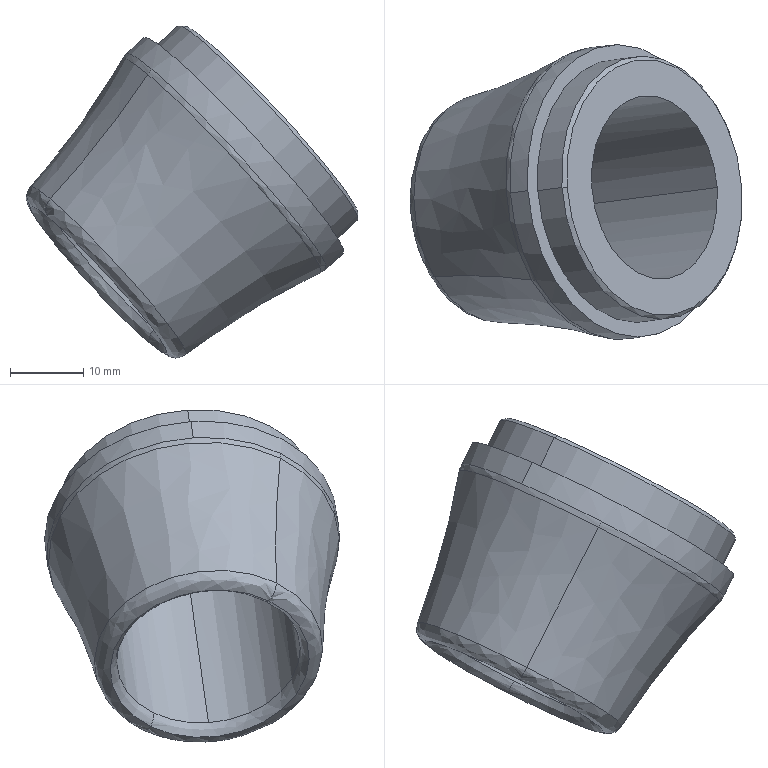Part | SolidWorks | features BaseBody 1 | 1 solid | 18 faces | box 45.199 x 40.143 x 45.272 mm | volume 15779 mm3 | spline 8 | cylinder 4 | cone 4 | plane 2 | commonest cylinder face diameters 25.135 x2 40 x2
STEP:
#1=CARTESIAN_POINT('',(673.604,-209.277,202.973));
#2=VERTEX_POINT('',#1);
#3=CARTESIAN_POINT('',(687.345,-193.141,185.868));
#4=VERTEX_POINT('',#3);
#5=CARTESIAN_POINT('',(680.475,-201.209,194.421));
#6=DIRECTION('',(-0.7306,-0.09465,-0.6762));
#7=DIRECTION('',(-0.5045,-0.5925,0.628));
#8=AXIS2_PLACEMENT_3D('',#5,#6,#7);
#9=CIRCLE('',#8,13.618);
#10=EDGE_CURVE('',#2,#4,#9,.T.);
#11=ORIENTED_EDGE('',*,*,#10,.T.);
#12=CARTESIAN_POINT('',(688.101,-193.596,187.718));
#13=VERTEX_POINT('',#12);
#14=CARTESIAN_POINT('',(689.111,-192.411,186.462));
#15=DIRECTION('',(-0.4601,0.8,0.3851));
#16=DIRECTION('',(0.5045,0.5925,-0.628));
#17=AXIS2_PLACEMENT_3D('',#14,#15,#16);
#18=CIRCLE('',#17,2.);
#19=EDGE_CURVE('',#4,#13,#18,.T.);
#20=ORIENTED_EDGE('',*,*,#19,.T.);
#21=CARTESIAN_POINT('',(673.224,-201.042,204.834));
#22=VERTEX_POINT('',#21);
#23=CARTESIAN_POINT('',(681.761,-201.042,195.611));
#24=DIRECTION('',(0.7306,0.09465,0.6762));
#25=DIRECTION('',(-0.6793,0.,0.7339));
#26=AXIS2_PLACEMENT_3D('',#23,#24,#25);
#27=CIRCLE('',#26,12.567);
#28=EDGE_CURVE('',#13,#22,#27,.T.);
#29=ORIENTED_EDGE('',*,*,#28,.T.);
#30=CARTESIAN_POINT('',(675.42,-208.488,203.504));
#31=VERTEX_POINT('',#30);
#32=CARTESIAN_POINT('',(681.761,-201.042,195.611));
#33=DIRECTION('',(0.7306,0.09465,0.6762));
#34=DIRECTION('',(-0.6793,0.,0.7339));
#35=AXIS2_PLACEMENT_3D('',#32,#33,#34);
#36=CIRCLE('',#35,12.567);
#37=EDGE_CURVE('',#22,#31,#36,.T.);
#38=ORIENTED_EDGE('',*,*,#37,.T.);
#39=CARTESIAN_POINT('',(674.411,-209.673,204.76));
#40=DIRECTION('',(0.4601,-0.8,-0.3851));
#41=DIRECTION('',(-0.5045,-0.5925,0.628));
#42=AXIS2_PLACEMENT_3D('',#39,#40,#41);
#43=CIRCLE('',#42,2.);
#44=EDGE_CURVE('',#2,#31,#43,.T.);
#45=ORIENTED_EDGE('',*,*,#44,.F.);
#46=EDGE_LOOP('',(#11,#20,#29,#38,#45));
#47=FACE_OUTER_BOUND('',#46,.T.);
#48=CARTESIAN_POINT('',(687.345,-193.141,185.868));
#49=CARTESIAN_POINT('',(674.815,-171.352,196.357));
#50=CARTESIAN_POINT('',(661.073,-187.488,213.462));
#51=CARTESIAN_POINT('',(673.604,-209.277,202.973));
#52=CARTESIAN_POINT('',(687.272,-193.5,186.527));
#53=CARTESIAN_POINT('',(675.352,-172.773,196.505));
#54=CARTESIAN_POINT('',(662.281,-188.123,212.776));
#55=CARTESIAN_POINT('',(674.201,-208.85,202.798));
#56=CARTESIAN_POINT('',(687.55,-193.668,187.208));
#57=CARTESIAN_POINT('',(675.986,-173.56,196.888));
#58=CARTESIAN_POINT('',(663.305,-188.451,212.673));
#59=CARTESIAN_POINT('',(674.869,-208.559,202.994));
#60=CARTESIAN_POINT('',(688.101,-193.596,187.718));
#61=CARTESIAN_POINT('',(676.537,-173.488,197.398));
#62=CARTESIAN_POINT('',(663.856,-188.38,213.183));
#63=CARTESIAN_POINT('',(675.42,-208.488,203.504));
#64=(BOUNDED_SURFACE()B_SPLINE_SURFACE(3,3,((#48,#49,#50,#51),(#52,#53,#54,#55),(#56,#57,#58,#59),(#60,#61,#62,#63)),.UNSPECIFIED.,.F.,.F.,.T.)B_SPLINE_SURFACE_WITH_KNOTS((4,4),(4,4),(0.,1.),(0.,1.),.UNSPECIFIED.)GEOMETRIC_REPRESENTATION_ITEM()RATIONAL_B_SPLINE_SURFACE(((1.,0.3333,0.3333,1.),(0.9058,0.3019,0.3019,0.9058),(0.9058,0.3019,0.3019,0.9058),(1.,0.3333,0.3333,1.)))REPRESENTATION_ITEM('')SURFACE());
#65=ADVANCED_FACE('',(#47),#64,.T.);
#66=CARTESIAN_POINT('',(673.91,-210.286,205.434));
#67=VERTEX_POINT('',#66);
#68=CARTESIAN_POINT('',(689.659,-191.792,185.831));
#69=VERTEX_POINT('',#68);
#70=CARTESIAN_POINT('',(681.784,-201.039,195.633));
#71=DIRECTION('',(-0.7306,-0.09465,-0.6762));
#72=DIRECTION('',(-0.5045,-0.5925,0.628));
#73=AXIS2_PLACEMENT_3D('',#70,#71,#72);
#74=CIRCLE('',#73,15.607);
#75=EDGE_CURVE('',#67,#69,#74,.T.);
#76=ORIENTED_EDGE('',*,*,#75,.T.);
#77=CARTESIAN_POINT('',(688.807,-192.951,187.221));
#78=DIRECTION('',(-0.4601,0.8,0.3851));
#79=DIRECTION('',(0.5045,0.5925,-0.628));
#80=AXIS2_PLACEMENT_3D('',#77,#78,#79);
#81=CIRCLE('',#80,2.);
#82=EDGE_CURVE('',#69,#4,#81,.T.);
#83=ORIENTED_EDGE('',*,*,#82,.T.);
#84=ORIENTED_EDGE('',*,*,#10,.F.);
#85=CARTESIAN_POINT('',(675.065,-209.088,204.326));
#86=DIRECTION('',(0.4601,-0.8,-0.3851));
#87=DIRECTION('',(-0.5045,-0.5925,0.628));
#88=AXIS2_PLACEMENT_3D('',#85,#86,#87);
#89=CIRCLE('',#88,2.);
#90=EDGE_CURVE('',#67,#2,#89,.T.);
#91=ORIENTED_EDGE('',*,*,#90,.F.);
#92=EDGE_LOOP('',(#76,#83,#84,#91));
#93=FACE_OUTER_BOUND('',#92,.T.);
#94=CARTESIAN_POINT('',(689.659,-191.792,185.831));
#95=CARTESIAN_POINT('',(675.297,-166.821,197.852));
#96=CARTESIAN_POINT('',(659.549,-185.314,217.455));
#97=CARTESIAN_POINT('',(673.91,-210.286,205.434));
#98=CARTESIAN_POINT('',(688.819,-191.96,185.177));
#99=CARTESIAN_POINT('',(674.561,-167.167,197.111));
#100=CARTESIAN_POINT('',(658.925,-185.528,216.574));
#101=CARTESIAN_POINT('',(673.183,-210.321,204.64));
#102=CARTESIAN_POINT('',(687.889,-192.502,185.192));
#103=CARTESIAN_POINT('',(674.367,-168.99,196.51));
#104=CARTESIAN_POINT('',(659.539,-186.403,214.968));
#105=CARTESIAN_POINT('',(673.06,-209.915,203.65));
#106=CARTESIAN_POINT('',(687.345,-193.141,185.868));
#107=CARTESIAN_POINT('',(674.815,-171.352,196.357));
#108=CARTESIAN_POINT('',(661.073,-187.488,213.462));
#109=CARTESIAN_POINT('',(673.604,-209.277,202.973));
#110=(BOUNDED_SURFACE()B_SPLINE_SURFACE(3,3,((#94,#95,#96,#97),(#98,#99,#100,#101),(#102,#103,#104,#105),(#106,#107,#108,#109)),.UNSPECIFIED.,.F.,.F.,.T.)B_SPLINE_SURFACE_WITH_KNOTS((4,4),(4,4),(0.,1.),(0.,1.),.UNSPECIFIED.)GEOMETRIC_REPRESENTATION_ITEM()RATIONAL_B_SPLINE_SURFACE(((1.,0.3333,0.3333,1.),(0.8286,0.2762,0.2762,0.8286),(0.8286,0.2762,0.2762,0.8286),(1.,0.3333,0.3333,1.)))REPRESENTATION_ITEM('')SURFACE());
#111=ADVANCED_FACE('',(#93),#110,.T.);
#112=CARTESIAN_POINT('',(681.784,-201.039,195.633));
#113=DIRECTION('',(-0.7306,-0.09465,-0.6762));
#114=DIRECTION('',(-0.5045,-0.5925,0.628));
#115=AXIS2_PLACEMENT_3D('',#112,#113,#114);
#116=CIRCLE('',#115,15.607);
#117=EDGE_CURVE('',#69,#67,#116,.T.);
#118=ORIENTED_EDGE('',*,*,#117,.F.);
#119=CARTESIAN_POINT('',(707.241,-187.267,197.437));
#120=VERTEX_POINT('',#119);
#121=CARTESIAN_POINT('',(737.952,-126.097,107.052));
#122=DIRECTION('',(-0.4601,0.8,0.3851));
#123=DIRECTION('',(0.5045,0.5925,-0.628));
#124=AXIS2_PLACEMENT_3D('',#121,#122,#123);
#125=CIRCLE('',#124,113.377);
#126=EDGE_CURVE('',#69,#120,#125,.T.);
#127=ORIENTED_EDGE('',*,*,#126,.T.);
#128=CARTESIAN_POINT('',(687.19,-210.813,222.396));
#129=VERTEX_POINT('',#128);
#130=CARTESIAN_POINT('',(697.216,-199.04,209.916));
#131=DIRECTION('',(0.7306,0.09465,0.6762));
#132=DIRECTION('',(-0.5045,-0.5925,0.628));
#133=AXIS2_PLACEMENT_3D('',#130,#131,#132);
#134=CIRCLE('',#133,19.871);
#135=EDGE_CURVE('',#129,#120,#134,.T.);
#136=ORIENTED_EDGE('',*,*,#135,.F.);
#137=CARTESIAN_POINT('',(608.416,-278.209,268.293));
#138=DIRECTION('',(0.4601,-0.8,-0.3851));
#139=DIRECTION('',(-0.5045,-0.5925,0.628));
#140=AXIS2_PLACEMENT_3D('',#137,#138,#139);
#141=CIRCLE('',#140,113.377);
#142=EDGE_CURVE('',#67,#129,#141,.T.);
#143=ORIENTED_EDGE('',*,*,#142,.F.);
#144=EDGE_LOOP('',(#118,#127,#136,#143));
#145=FACE_OUTER_BOUND('',#144,.T.);
#146=CARTESIAN_POINT('',(673.91,-210.286,205.434));
#147=CARTESIAN_POINT('',(688.271,-235.258,193.414));
#148=CARTESIAN_POINT('',(704.02,-216.764,173.81));
#149=CARTESIAN_POINT('',(689.659,-191.792,185.831));
#150=CARTESIAN_POINT('',(678.767,-210.051,210.75));
#151=CARTESIAN_POINT('',(693.817,-236.22,198.153));
#152=CARTESIAN_POINT('',(710.32,-216.84,177.61));
#153=CARTESIAN_POINT('',(695.271,-190.671,190.207));
#154=CARTESIAN_POINT('',(683.208,-210.227,216.421));
#155=CARTESIAN_POINT('',(699.569,-238.677,202.726));
#156=CARTESIAN_POINT('',(717.511,-217.608,180.392));
#157=CARTESIAN_POINT('',(701.15,-189.158,194.087));
#158=CARTESIAN_POINT('',(687.19,-210.813,222.396));
#159=CARTESIAN_POINT('',(705.475,-242.607,207.091));
#160=CARTESIAN_POINT('',(725.526,-219.061,182.132));
#161=CARTESIAN_POINT('',(707.241,-187.267,197.437));
#162=(BOUNDED_SURFACE()B_SPLINE_SURFACE(3,3,((#146,#147,#148,#149),(#150,#151,#152,#153),(#154,#155,#156,#157),(#158,#159,#160,#161)),.UNSPECIFIED.,.F.,.F.,.T.)B_SPLINE_SURFACE_WITH_KNOTS((4,4),(4,4),(0.,1.),(0.,1.),.UNSPECIFIED.)GEOMETRIC_REPRESENTATION_ITEM()RATIONAL_B_SPLINE_SURFACE(((1.,0.3333,0.3333,1.),(0.997,0.3323,0.3323,0.997),(0.997,0.3323,0.3323,0.997),(1.,0.3333,0.3333,1.)))REPRESENTATION_ITEM('')SURFACE());
#163=ADVANCED_FACE('',(#145),#162,.F.);
#164=CARTESIAN_POINT('',(684.266,-198.958,225.182));
#165=VERTEX_POINT('',#164);
#166=CARTESIAN_POINT('',(707.942,-187.108,197.944));
#167=VERTEX_POINT('',#166);
#168=CARTESIAN_POINT('',(697.852,-198.958,210.505));
#169=DIRECTION('',(-0.7306,-0.09465,-0.6762));
#170=DIRECTION('',(-0.5045,-0.5925,0.628));
#171=AXIS2_PLACEMENT_3D('',#168,#169,#170);
#172=CIRCLE('',#171,20.);
#173=EDGE_CURVE('',#165,#167,#172,.T.);
#174=ORIENTED_EDGE('',*,*,#173,.T.);
#175=CARTESIAN_POINT('',(706.429,-188.886,199.828));
#176=DIRECTION('',(-0.4601,0.8,0.3851));
#177=DIRECTION('',(0.5045,0.5925,-0.628));
#178=AXIS2_PLACEMENT_3D('',#175,#176,#177);
#179=CIRCLE('',#178,3.);
#180=EDGE_CURVE('',#167,#120,#179,.T.);
#181=ORIENTED_EDGE('',*,*,#180,.T.);
#182=CARTESIAN_POINT('',(697.216,-199.04,209.916));
#183=DIRECTION('',(0.7306,0.09465,0.6762));
#184=DIRECTION('',(-0.5045,-0.5925,0.628));
#185=AXIS2_PLACEMENT_3D('',#182,#183,#184);
#186=CIRCLE('',#185,19.871);
#187=EDGE_CURVE('',#120,#129,#186,.T.);
#188=ORIENTED_EDGE('',*,*,#187,.T.);
#189=CARTESIAN_POINT('',(687.761,-210.807,223.065));
#190=VERTEX_POINT('',#189);
#191=CARTESIAN_POINT('',(689.275,-209.03,221.181));
#192=DIRECTION('',(0.4601,-0.8,-0.3851));
#193=DIRECTION('',(-0.5045,-0.5925,0.628));
#194=AXIS2_PLACEMENT_3D('',#191,#192,#193);
#195=CIRCLE('',#194,3.);
#196=EDGE_CURVE('',#190,#129,#195,.T.);
#197=ORIENTED_EDGE('',*,*,#196,.F.);
#198=CARTESIAN_POINT('',(697.852,-198.958,210.505));
#199=DIRECTION('',(-0.7306,-0.09465,-0.6762));
#200=DIRECTION('',(-0.5045,-0.5925,0.628));
#201=AXIS2_PLACEMENT_3D('',#198,#199,#200);
#202=CIRCLE('',#201,20.);
#203=EDGE_CURVE('',#190,#165,#202,.T.);
#204=ORIENTED_EDGE('',*,*,#203,.T.);
#205=EDGE_LOOP('',(#174,#181,#188,#197,#204));
#206=FACE_OUTER_BOUND('',#205,.T.);
#207=CARTESIAN_POINT('',(707.942,-187.108,197.944));
#208=CARTESIAN_POINT('',(689.539,-155.108,213.348));
#209=CARTESIAN_POINT('',(669.358,-178.806,238.469));
#210=CARTESIAN_POINT('',(687.761,-210.807,223.065));
#211=CARTESIAN_POINT('',(707.727,-187.136,197.744));
#212=CARTESIAN_POINT('',(689.323,-155.136,213.148));
#213=CARTESIAN_POINT('',(669.142,-178.834,238.269));
#214=CARTESIAN_POINT('',(687.545,-210.835,222.865));
#215=CARTESIAN_POINT('',(707.491,-187.19,197.574));
#216=CARTESIAN_POINT('',(689.128,-155.258,212.944));
#217=CARTESIAN_POINT('',(668.99,-178.906,238.011));
#218=CARTESIAN_POINT('',(687.353,-210.837,222.641));
#219=CARTESIAN_POINT('',(707.241,-187.267,197.437));
#220=CARTESIAN_POINT('',(688.957,-155.473,212.741));
#221=CARTESIAN_POINT('',(668.906,-179.019,237.7));
#222=CARTESIAN_POINT('',(687.19,-210.813,222.396));
#223=(BOUNDED_SURFACE()B_SPLINE_SURFACE(3,3,((#207,#208,#209,#210),(#211,#212,#213,#214),(#215,#216,#217,#218),(#219,#220,#221,#222)),.UNSPECIFIED.,.F.,.F.,.F.)B_SPLINE_SURFACE_WITH_KNOTS((4,4),(4,4),(0.,1.),(0.,1.),.UNSPECIFIED.)GEOMETRIC_REPRESENTATION_ITEM()RATIONAL_B_SPLINE_SURFACE(((1.,0.3333,0.3333,1.),(0.9928,0.3309,0.3309,0.9928),(0.9928,0.3309,0.3309,0.9928),(1.,0.3333,0.3333,1.)))REPRESENTATION_ITEM('')SURFACE());
#224=ADVANCED_FACE('',(#206),#223,.T.);
#225=CARTESIAN_POINT('',(712.424,-198.176,206.868));
#226=VERTEX_POINT('',#225);
#227=CARTESIAN_POINT('',(695.351,-198.176,225.314));
#228=VERTEX_POINT('',#227);
#229=CARTESIAN_POINT('',(703.887,-198.176,216.091));
#230=DIRECTION('',(-0.7306,-0.09465,-0.6762));
#231=DIRECTION('',(-0.6793,0.,0.7339));
#232=AXIS2_PLACEMENT_3D('',#229,#230,#231);
#233=CIRCLE('',#232,12.567);
#234=EDGE_CURVE('',#226,#228,#233,.T.);
#235=ORIENTED_EDGE('',*,*,#234,.F.);
#236=CARTESIAN_POINT('',(690.297,-201.042,186.388));
#237=VERTEX_POINT('',#236);
#238=CARTESIAN_POINT('',(689.011,-201.209,185.198));
#239=DIRECTION('',(-0.7306,-0.09465,-0.6762));
#240=VECTOR('',#239,1000.);
#241=LINE('',#238,#240);
#242=EDGE_CURVE('',#226,#237,#241,.T.);
#243=ORIENTED_EDGE('',*,*,#242,.T.);
#244=CARTESIAN_POINT('',(681.761,-201.042,195.611));
#245=DIRECTION('',(0.7306,0.09465,0.6762));
#246=DIRECTION('',(-0.6793,0.,0.7339));
#247=AXIS2_PLACEMENT_3D('',#244,#245,#246);
#248=CIRCLE('',#247,12.567);
#249=EDGE_CURVE('',#31,#237,#248,.T.);
#250=ORIENTED_EDGE('',*,*,#249,.F.);
#251=ORIENTED_EDGE('',*,*,#37,.F.);
#252=CARTESIAN_POINT('',(671.938,-201.209,203.644));
#253=DIRECTION('',(-0.7306,-0.09465,-0.6762));
#254=VECTOR('',#253,1000.);
#255=LINE('',#252,#254);
#256=EDGE_CURVE('',#228,#22,#255,.T.);
#257=ORIENTED_EDGE('',*,*,#256,.F.);
#258=EDGE_LOOP('',(#235,#243,#250,#251,#257));
#259=FACE_OUTER_BOUND('',#258,.T.);
#260=CARTESIAN_POINT('',(680.475,-201.209,194.421));
#261=DIRECTION('',(-0.7306,-0.09465,-0.6762));
#262=DIRECTION('',(-0.6793,0.,0.7339));
#263=AXIS2_PLACEMENT_3D('',#260,#261,#262);
#264=CYLINDRICAL_SURFACE('',#263,12.567);
#265=ADVANCED_FACE('',(#259),#264,.F.);
#266=CARTESIAN_POINT('',(715.774,-198.176,203.249));
#267=VERTEX_POINT('',#266);
#268=CARTESIAN_POINT('',(692.001,-198.176,228.934));
#269=VERTEX_POINT('',#268);
#270=CARTESIAN_POINT('',(703.887,-198.176,216.091));
#271=DIRECTION('',(0.7306,0.09465,0.6762));
#272=DIRECTION('',(-0.6793,0.,0.7339));
#273=AXIS2_PLACEMENT_3D('',#270,#271,#272);
#274=CIRCLE('',#273,17.499);
#275=EDGE_CURVE('',#267,#269,#274,.T.);
#276=ORIENTED_EDGE('',*,*,#275,.F.);
#277=CARTESIAN_POINT('',(715.749,-198.223,202.544));
#278=VERTEX_POINT('',#277);
#279=CARTESIAN_POINT('',(715.749,-198.223,202.544));
#280=DIRECTION('',(-0.0362,-0.06692,-0.9971));
#281=VECTOR('',#280,1000.);
#282=LINE('',#279,#281);
#283=EDGE_CURVE('',#267,#278,#282,.T.);
#284=ORIENTED_EDGE('',*,*,#283,.T.);
#285=CARTESIAN_POINT('',(691.296,-198.223,228.962));
#286=VERTEX_POINT('',#285);
#287=CARTESIAN_POINT('',(703.522,-198.223,215.753));
#288=DIRECTION('',(0.7306,0.09465,0.6762));
#289=DIRECTION('',(0.5045,0.5925,-0.628));
#290=AXIS2_PLACEMENT_3D('',#287,#288,#289);
#291=CIRCLE('',#290,17.999);
#292=EDGE_CURVE('',#278,#286,#291,.T.);
#293=ORIENTED_EDGE('',*,*,#292,.T.);
#294=CARTESIAN_POINT('',(691.296,-198.223,228.962));
#295=DIRECTION('',(-0.9969,-0.06692,0.04086));
#296=VECTOR('',#295,1000.);
#297=LINE('',#294,#296);
#298=EDGE_CURVE('',#269,#286,#297,.T.);
#299=ORIENTED_EDGE('',*,*,#298,.F.);
#300=EDGE_LOOP('',(#276,#284,#293,#299));
#301=FACE_OUTER_BOUND('',#300,.T.);
#302=CARTESIAN_POINT('',(703.522,-198.223,215.753));
#303=DIRECTION('',(-0.7306,-0.09465,-0.6762));
#304=DIRECTION('',(-0.6793,0.,0.7339));
#305=AXIS2_PLACEMENT_3D('',#302,#303,#304);
#306=CONICAL_SURFACE('',#305,17.999,0.7855);
#307=ADVANCED_FACE('',(#301),#306,.T.);
#308=ORIENTED_EDGE('',*,*,#292,.F.);
#309=CARTESIAN_POINT('',(712.461,-198.649,199.5));
#310=VERTEX_POINT('',#309);
#311=CARTESIAN_POINT('',(712.461,-198.649,199.5));
#312=DIRECTION('',(-0.7305,-0.09465,-0.6764));
#313=VECTOR('',#312,1000.);
#314=LINE('',#311,#313);
#315=EDGE_CURVE('',#278,#310,#314,.T.);
#316=ORIENTED_EDGE('',*,*,#315,.T.);
#317=CARTESIAN_POINT('',(688.008,-198.649,225.92));
#318=VERTEX_POINT('',#317);
#319=CARTESIAN_POINT('',(700.235,-198.649,212.71));
#320=DIRECTION('',(0.7306,0.09465,0.6762));
#321=DIRECTION('',(-0.6793,0.,0.7339));
#322=AXIS2_PLACEMENT_3D('',#319,#320,#321);
#323=CIRCLE('',#322,18.);
#324=EDGE_CURVE('',#310,#318,#323,.T.);
#325=ORIENTED_EDGE('',*,*,#324,.T.);
#326=CARTESIAN_POINT('',(688.008,-198.649,225.92));
#327=DIRECTION('',(-0.7307,-0.09465,-0.6761));
#328=VECTOR('',#327,1000.);
#329=LINE('',#326,#328);
#330=EDGE_CURVE('',#286,#318,#329,.T.);
#331=ORIENTED_EDGE('',*,*,#330,.F.);
#332=EDGE_LOOP('',(#308,#316,#325,#331));
#333=FACE_OUTER_BOUND('',#332,.T.);
#334=CARTESIAN_POINT('',(700.235,-198.649,212.71));
#335=DIRECTION('',(-0.7306,-0.09465,-0.6762));
#336=DIRECTION('',(-0.6793,0.,0.7339));
#337=AXIS2_PLACEMENT_3D('',#334,#335,#336);
#338=CONICAL_SURFACE('',#337,18.,0.0001745);
#339=ADVANCED_FACE('',(#333),#338,.T.);
#340=ORIENTED_EDGE('',*,*,#173,.F.);
#341=CARTESIAN_POINT('',(686.649,-198.649,227.388));
#342=VERTEX_POINT('',#341);
#343=CARTESIAN_POINT('',(685.294,-198.824,226.134));
#344=DIRECTION('',(0.7306,0.09465,0.6762));
#345=VECTOR('',#344,1000.);
#346=LINE('',#343,#345);
#347=EDGE_CURVE('',#165,#342,#346,.T.);
#348=ORIENTED_EDGE('',*,*,#347,.T.);
#349=CARTESIAN_POINT('',(713.82,-198.649,198.032));
#350=VERTEX_POINT('',#349);
#351=CARTESIAN_POINT('',(700.235,-198.649,212.71));
#352=DIRECTION('',(0.7306,0.09465,0.6762));
#353=DIRECTION('',(0.6793,0.,-0.7339));
#354=AXIS2_PLACEMENT_3D('',#351,#352,#353);
#355=CIRCLE('',#354,20.);
#356=EDGE_CURVE('',#350,#342,#355,.T.);
#357=ORIENTED_EDGE('',*,*,#356,.F.);
#358=CARTESIAN_POINT('',(711.437,-198.958,195.827));
#359=VERTEX_POINT('',#358);
#360=CARTESIAN_POINT('',(712.465,-198.824,196.778));
#361=DIRECTION('',(0.7306,0.09465,0.6762));
#362=VECTOR('',#361,1000.);
#363=LINE('',#360,#362);
#364=EDGE_CURVE('',#359,#350,#363,.T.);
#365=ORIENTED_EDGE('',*,*,#364,.F.);
#366=CARTESIAN_POINT('',(697.852,-198.958,210.505));
#367=DIRECTION('',(-0.7306,-0.09465,-0.6762));
#368=DIRECTION('',(-0.5045,-0.5925,0.628));
#369=AXIS2_PLACEMENT_3D('',#366,#367,#368);
#370=CIRCLE('',#369,20.);
#371=EDGE_CURVE('',#167,#359,#370,.T.);
#372=ORIENTED_EDGE('',*,*,#371,.F.);
#373=EDGE_LOOP('',(#340,#348,#357,#365,#372));
#374=FACE_OUTER_BOUND('',#373,.T.);
#375=CARTESIAN_POINT('',(698.88,-198.824,211.456));
#376=DIRECTION('',(0.7306,0.09465,0.6762));
#377=DIRECTION('',(0.6793,0.,-0.7339));
#378=AXIS2_PLACEMENT_3D('',#375,#376,#377);
#379=CYLINDRICAL_SURFACE('',#378,20.);
#380=ADVANCED_FACE('',(#374),#379,.T.);
#381=ORIENTED_EDGE('',*,*,#242,.F.);
#382=CARTESIAN_POINT('',(703.887,-198.176,216.091));
#383=DIRECTION('',(-0.7306,-0.09465,-0.6762));
#384=DIRECTION('',(-0.6793,0.,0.7339));
#385=AXIS2_PLACEMENT_3D('',#382,#383,#384);
#386=CIRCLE('',#385,12.567);
#387=EDGE_CURVE('',#228,#226,#386,.T.);
#388=ORIENTED_EDGE('',*,*,#387,.F.);
#389=ORIENTED_EDGE('',*,*,#256,.T.);
#390=ORIENTED_EDGE('',*,*,#28,.F.);
#391=CARTESIAN_POINT('',(681.761,-201.042,195.611));
#392=DIRECTION('',(0.7306,0.09465,0.6762));
#393=DIRECTION('',(-0.6793,0.,0.7339));
#394=AXIS2_PLACEMENT_3D('',#391,#392,#393);
#395=CIRCLE('',#394,12.567);
#396=EDGE_CURVE('',#237,#13,#395,.T.);
#397=ORIENTED_EDGE('',*,*,#396,.F.);
#398=EDGE_LOOP('',(#381,#388,#389,#390,#397));
#399=FACE_OUTER_BOUND('',#398,.T.);
#400=CARTESIAN_POINT('',(680.475,-201.209,194.421));
#401=DIRECTION('',(-0.7306,-0.09465,-0.6762));
#402=DIRECTION('',(-0.6793,0.,0.7339));
#403=AXIS2_PLACEMENT_3D('',#400,#401,#402);
#404=CYLINDRICAL_SURFACE('',#403,12.567);
#405=ADVANCED_FACE('',(#399),#404,.F.);
#406=CARTESIAN_POINT('',(703.887,-198.176,216.091));
#407=DIRECTION('',(0.7306,0.09465,0.6762));
#408=DIRECTION('',(-0.6793,0.,0.7339));
#409=AXIS2_PLACEMENT_3D('',#406,#407,#408);
#410=CIRCLE('',#409,17.499);
#411=EDGE_CURVE('',#269,#267,#410,.T.);
#412=ORIENTED_EDGE('',*,*,#411,.T.);
#413=ORIENTED_EDGE('',*,*,#275,.T.);
#414=EDGE_LOOP('',(#412,#413));
#415=FACE_OUTER_BOUND('',#414,.T.);
#416=ORIENTED_EDGE('',*,*,#387,.T.);
#417=ORIENTED_EDGE('',*,*,#234,.T.);
#418=EDGE_LOOP('',(#416,#417));
#419=FACE_BOUND('',#418,.T.);
#420=CARTESIAN_POINT('',(703.887,-198.176,216.091));
#421=DIRECTION('',(0.7306,0.09465,0.6762));
#422=DIRECTION('',(0.6793,0.,-0.7339));
#423=AXIS2_PLACEMENT_3D('',#420,#421,#422);
#424=PLANE('',#423);
#425=ADVANCED_FACE('',(#415,#419),#424,.T.);
#426=ORIENTED_EDGE('',*,*,#19,.F.);
#427=CARTESIAN_POINT('',(680.475,-201.209,194.421));
#428=DIRECTION('',(-0.7306,-0.09465,-0.6762));
#429=DIRECTION('',(-0.5045,-0.5925,0.628));
#430=AXIS2_PLACEMENT_3D('',#427,#428,#429);
#431=CIRCLE('',#430,13.618);
#432=EDGE_CURVE('',#4,#2,#431,.T.);
#433=ORIENTED_EDGE('',*,*,#432,.T.);
#434=ORIENTED_EDGE('',*,*,#44,.T.);
#435=ORIENTED_EDGE('',*,*,#249,.T.);
#436=ORIENTED_EDGE('',*,*,#396,.T.);
#437=EDGE_LOOP('',(#426,#433,#434,#435,#436));
#438=FACE_OUTER_BOUND('',#437,.T.);
#439=CARTESIAN_POINT('',(673.604,-209.277,202.973));
#440=CARTESIAN_POINT('',(686.135,-231.066,192.485));
#441=CARTESIAN_POINT('',(699.876,-214.93,175.38));
#442=CARTESIAN_POINT('',(687.345,-193.141,185.868));
#443=CARTESIAN_POINT('',(674.201,-208.85,202.798));
#444=CARTESIAN_POINT('',(686.12,-229.577,192.821));
#445=CARTESIAN_POINT('',(699.192,-214.227,176.55));
#446=CARTESIAN_POINT('',(687.272,-193.5,186.527));
#447=CARTESIAN_POINT('',(674.869,-208.559,202.994));
#448=CARTESIAN_POINT('',(686.433,-228.668,193.314));
#449=CARTESIAN_POINT('',(699.114,-213.776,177.529));
#450=CARTESIAN_POINT('',(687.55,-193.668,187.208));
#451=CARTESIAN_POINT('',(675.42,-208.488,203.504));
#452=CARTESIAN_POINT('',(686.984,-228.596,193.824));
#453=CARTESIAN_POINT('',(699.666,-213.705,178.039));
#454=CARTESIAN_POINT('',(688.101,-193.596,187.718));
#455=(BOUNDED_SURFACE()B_SPLINE_SURFACE(3,3,((#439,#440,#441,#442),(#443,#444,#445,#446),(#447,#448,#449,#450),(#451,#452,#453,#454)),.UNSPECIFIED.,.F.,.F.,.T.)B_SPLINE_SURFACE_WITH_KNOTS((4,4),(4,4),(0.,1.),(0.,1.),.UNSPECIFIED.)GEOMETRIC_REPRESENTATION_ITEM()RATIONAL_B_SPLINE_SURFACE(((1.,0.3333,0.3333,1.),(0.9058,0.3019,0.3019,0.9058),(0.9058,0.3019,0.3019,0.9058),(1.,0.3333,0.3333,1.)))REPRESENTATION_ITEM('')SURFACE());
#456=ADVANCED_FACE('',(#438),#455,.T.);
#457=ORIENTED_EDGE('',*,*,#283,.F.);
#458=ORIENTED_EDGE('',*,*,#411,.F.);
#459=ORIENTED_EDGE('',*,*,#298,.T.);
#460=CARTESIAN_POINT('',(703.522,-198.223,215.753));
#461=DIRECTION('',(0.7306,0.09465,0.6762));
#462=DIRECTION('',(0.5045,0.5925,-0.628));
#463=AXIS2_PLACEMENT_3D('',#460,#461,#462);
#464=CIRCLE('',#463,17.999);
#465=EDGE_CURVE('',#286,#278,#464,.T.);
#466=ORIENTED_EDGE('',*,*,#465,.T.);
#467=EDGE_LOOP('',(#457,#458,#459,#466));
#468=FACE_OUTER_BOUND('',#467,.T.);
#469=CARTESIAN_POINT('',(703.522,-198.223,215.753));
#470=DIRECTION('',(-0.7306,-0.09465,-0.6762));
#471=DIRECTION('',(-0.6793,0.,0.7339));
#472=AXIS2_PLACEMENT_3D('',#469,#470,#471);
#473=CONICAL_SURFACE('',#472,17.999,0.7855);
#474=ADVANCED_FACE('',(#468),#473,.T.);
#475=ORIENTED_EDGE('',*,*,#82,.F.);
#476=ORIENTED_EDGE('',*,*,#117,.T.);
#477=ORIENTED_EDGE('',*,*,#90,.T.);
#478=ORIENTED_EDGE('',*,*,#432,.F.);
#479=EDGE_LOOP('',(#475,#476,#477,#478));
#480=FACE_OUTER_BOUND('',#479,.T.);
#481=CARTESIAN_POINT('',(673.91,-210.286,205.434));
#482=CARTESIAN_POINT('',(688.271,-235.258,193.414));
#483=CARTESIAN_POINT('',(704.02,-216.764,173.81));
#484=CARTESIAN_POINT('',(689.659,-191.792,185.831));
#485=CARTESIAN_POINT('',(673.183,-210.321,204.64));
#486=CARTESIAN_POINT('',(687.442,-235.114,192.705));
#487=CARTESIAN_POINT('',(703.078,-216.753,173.242));
#488=CARTESIAN_POINT('',(688.819,-191.96,185.177));
#489=CARTESIAN_POINT('',(673.06,-209.915,203.65));
#490=CARTESIAN_POINT('',(686.582,-233.428,192.331));
#491=CARTESIAN_POINT('',(701.411,-216.015,173.874));
#492=CARTESIAN_POINT('',(687.889,-192.502,185.192));
#493=CARTESIAN_POINT('',(673.604,-209.277,202.973));
#494=CARTESIAN_POINT('',(686.135,-231.066,192.485));
#495=CARTESIAN_POINT('',(699.876,-214.93,175.38));
#496=CARTESIAN_POINT('',(687.345,-193.141,185.868));
#497=(BOUNDED_SURFACE()B_SPLINE_SURFACE(3,3,((#481,#482,#483,#484),(#485,#486,#487,#488),(#489,#490,#491,#492),(#493,#494,#495,#496)),.UNSPECIFIED.,.F.,.F.,.T.)B_SPLINE_SURFACE_WITH_KNOTS((4,4),(4,4),(0.,1.),(0.,1.),.UNSPECIFIED.)GEOMETRIC_REPRESENTATION_ITEM()RATIONAL_B_SPLINE_SURFACE(((1.,0.3333,0.3333,1.),(0.8286,0.2762,0.2762,0.8286),(0.8286,0.2762,0.2762,0.8286),(1.,0.3333,0.3333,1.)))REPRESENTATION_ITEM('')SURFACE());
#498=ADVANCED_FACE('',(#480),#497,.T.);
#499=ORIENTED_EDGE('',*,*,#315,.F.);
#500=ORIENTED_EDGE('',*,*,#465,.F.);
#501=ORIENTED_EDGE('',*,*,#330,.T.);
#502=CARTESIAN_POINT('',(700.235,-198.649,212.71));
#503=DIRECTION('',(0.7306,0.09465,0.6762));
#504=DIRECTION('',(-0.6793,0.,0.7339));
#505=AXIS2_PLACEMENT_3D('',#502,#503,#504);
#506=CIRCLE('',#505,18.);
#507=EDGE_CURVE('',#318,#310,#506,.T.);
#508=ORIENTED_EDGE('',*,*,#507,.T.);
#509=EDGE_LOOP('',(#499,#500,#501,#508));
#510=FACE_OUTER_BOUND('',#509,.T.);
#511=CARTESIAN_POINT('',(700.235,-198.649,212.71));
#512=DIRECTION('',(-0.7306,-0.09465,-0.6762));
#513=DIRECTION('',(-0.6793,0.,0.7339));
#514=AXIS2_PLACEMENT_3D('',#511,#512,#513);
#515=CONICAL_SURFACE('',#514,18.,0.0001745);
#516=ADVANCED_FACE('',(#510),#515,.T.);
#517=ORIENTED_EDGE('',*,*,#126,.F.);
#518=ORIENTED_EDGE('',*,*,#75,.F.);
#519=ORIENTED_EDGE('',*,*,#142,.T.);
#520=ORIENTED_EDGE('',*,*,#187,.F.);
#521=EDGE_LOOP('',(#517,#518,#519,#520));
#522=FACE_OUTER_BOUND('',#521,.T.);
#523=CARTESIAN_POINT('',(689.659,-191.792,185.831));
#524=CARTESIAN_POINT('',(675.297,-166.821,197.852));
#525=CARTESIAN_POINT('',(659.549,-185.314,217.455));
#526=CARTESIAN_POINT('',(673.91,-210.286,205.434));
#527=CARTESIAN_POINT('',(695.271,-190.671,190.207));
#528=CARTESIAN_POINT('',(680.222,-164.502,202.803));
#529=CARTESIAN_POINT('',(663.718,-183.882,223.346));
#530=CARTESIAN_POINT('',(678.767,-210.051,210.75));
#531=CARTESIAN_POINT('',(701.15,-189.158,194.087));
#532=CARTESIAN_POINT('',(684.789,-160.708,207.782));
#533=CARTESIAN_POINT('',(666.846,-181.777,230.115));
#534=CARTESIAN_POINT('',(683.208,-210.227,216.421));
#535=CARTESIAN_POINT('',(707.241,-187.267,197.437));
#536=CARTESIAN_POINT('',(688.957,-155.473,212.741));
#537=CARTESIAN_POINT('',(668.906,-179.019,237.7));
#538=CARTESIAN_POINT('',(687.19,-210.813,222.396));
#539=(BOUNDED_SURFACE()B_SPLINE_SURFACE(3,3,((#523,#524,#525,#526),(#527,#528,#529,#530),(#531,#532,#533,#534),(#535,#536,#537,#538)),.UNSPECIFIED.,.F.,.F.,.T.)B_SPLINE_SURFACE_WITH_KNOTS((4,4),(4,4),(0.,1.),(0.,1.),.UNSPECIFIED.)GEOMETRIC_REPRESENTATION_ITEM()RATIONAL_B_SPLINE_SURFACE(((1.,0.3333,0.3333,1.),(0.997,0.3323,0.3323,0.997),(0.997,0.3323,0.3323,0.997),(1.,0.3333,0.3333,1.)))REPRESENTATION_ITEM('')SURFACE());
#540=ADVANCED_FACE('',(#522),#539,.F.);
#541=ORIENTED_EDGE('',*,*,#507,.F.);
#542=ORIENTED_EDGE('',*,*,#324,.F.);
#543=EDGE_LOOP('',(#541,#542));
#544=FACE_BOUND('',#543,.T.);
#545=ORIENTED_EDGE('',*,*,#356,.T.);
#546=CARTESIAN_POINT('',(700.235,-198.649,212.71));
#547=DIRECTION('',(0.7306,0.09465,0.6762));
#548=DIRECTION('',(0.6793,0.,-0.7339));
#549=AXIS2_PLACEMENT_3D('',#546,#547,#548);
#550=CIRCLE('',#549,20.);
#551=EDGE_CURVE('',#342,#350,#550,.T.);
#552=ORIENTED_EDGE('',*,*,#551,.T.);
#553=EDGE_LOOP('',(#545,#552));
#554=FACE_OUTER_BOUND('',#553,.T.);
#555=CARTESIAN_POINT('',(695.189,-204.574,218.99));
#556=DIRECTION('',(0.7306,0.09465,0.6762));
#557=DIRECTION('',(0.6793,0.,-0.7339));
#558=AXIS2_PLACEMENT_3D('',#555,#556,#557);
#559=PLANE('',#558);
#560=ADVANCED_FACE('',(#544,#554),#559,.T.);
#561=ORIENTED_EDGE('',*,*,#180,.F.);
#562=ORIENTED_EDGE('',*,*,#371,.T.);
#563=CARTESIAN_POINT('',(697.852,-198.958,210.505));
#564=DIRECTION('',(-0.7306,-0.09465,-0.6762));
#565=DIRECTION('',(-0.5045,-0.5925,0.628));
#566=AXIS2_PLACEMENT_3D('',#563,#564,#565);
#567=CIRCLE('',#566,20.);
#568=EDGE_CURVE('',#359,#190,#567,.T.);
#569=ORIENTED_EDGE('',*,*,#568,.T.);
#570=ORIENTED_EDGE('',*,*,#196,.T.);
#571=ORIENTED_EDGE('',*,*,#135,.T.);
#572=EDGE_LOOP('',(#561,#562,#569,#570,#571));
#573=FACE_OUTER_BOUND('',#572,.T.);
#574=CARTESIAN_POINT('',(687.761,-210.807,223.065));
#575=CARTESIAN_POINT('',(706.164,-242.808,207.661));
#576=CARTESIAN_POINT('',(726.346,-219.109,182.54));
#577=CARTESIAN_POINT('',(707.942,-187.108,197.944));
#578=CARTESIAN_POINT('',(687.545,-210.835,222.865));
#579=CARTESIAN_POINT('',(705.948,-242.836,207.461));
#580=CARTESIAN_POINT('',(726.13,-219.137,182.34));
#581=CARTESIAN_POINT('',(707.727,-187.136,197.744));
#582=CARTESIAN_POINT('',(687.353,-210.837,222.641));
#583=CARTESIAN_POINT('',(705.717,-242.768,207.27));
#584=CARTESIAN_POINT('',(725.855,-219.121,182.203));
#585=CARTESIAN_POINT('',(707.491,-187.19,197.574));
#586=CARTESIAN_POINT('',(687.19,-210.813,222.396));
#587=CARTESIAN_POINT('',(705.475,-242.607,207.091));
#588=CARTESIAN_POINT('',(725.526,-219.061,182.132));
#589=CARTESIAN_POINT('',(707.241,-187.267,197.437));
#590=(BOUNDED_SURFACE()B_SPLINE_SURFACE(3,3,((#574,#575,#576,#577),(#578,#579,#580,#581),(#582,#583,#584,#585),(#586,#587,#588,#589)),.UNSPECIFIED.,.F.,.F.,.F.)B_SPLINE_SURFACE_WITH_KNOTS((4,4),(4,4),(0.,1.),(0.,1.),.UNSPECIFIED.)GEOMETRIC_REPRESENTATION_ITEM()RATIONAL_B_SPLINE_SURFACE(((1.,0.3333,0.3333,1.),(0.9928,0.3309,0.3309,0.9928),(0.9928,0.3309,0.3309,0.9928),(1.,0.3333,0.3333,1.)))REPRESENTATION_ITEM('')SURFACE());
#591=ADVANCED_FACE('',(#573),#590,.T.);
#592=ORIENTED_EDGE('',*,*,#347,.F.);
#593=ORIENTED_EDGE('',*,*,#203,.F.);
#594=ORIENTED_EDGE('',*,*,#568,.F.);
#595=ORIENTED_EDGE('',*,*,#364,.T.);
#596=ORIENTED_EDGE('',*,*,#551,.F.);
#597=EDGE_LOOP('',(#592,#593,#594,#595,#596));
#598=FACE_OUTER_BOUND('',#597,.T.);
#599=CARTESIAN_POINT('',(698.88,-198.824,211.456));
#600=DIRECTION('',(0.7306,0.09465,0.6762));
#601=DIRECTION('',(0.6793,0.,-0.7339));
#602=AXIS2_PLACEMENT_3D('',#599,#600,#601);
#603=CYLINDRICAL_SURFACE('',#602,20.);
#604=ADVANCED_FACE('',(#598),#603,.T.);
#605=CLOSED_SHELL('',(#65,#111,#163,#224,#265,#307,#339,#380,#405,#425,#456,#474,#498,#516,#540,#560,#591,#604));
#606=MANIFOLD_SOLID_BREP('',#605);
#607=CARTESIAN_POINT('',(0.,0.,0.));
#608=DIRECTION('',(0.,0.,1.));
#609=DIRECTION('',(1.,0.,0.));
#610=AXIS2_PLACEMENT_3D('',#607,#608,#609);
#611=(LENGTH_UNIT()NAMED_UNIT(*)SI_UNIT(.MILLI.,.METRE.));
#612=UNCERTAINTY_MEASURE_WITH_UNIT(LENGTH_MEASURE(0.00001),#611,'','');
#613=(NAMED_UNIT(*)PLANE_ANGLE_UNIT()SI_UNIT($,.RADIAN.));
#614=(NAMED_UNIT(*)SI_UNIT($,.STERADIAN.)SOLID_ANGLE_UNIT());
#615=(GEOMETRIC_REPRESENTATION_CONTEXT(3)GLOBAL_UNCERTAINTY_ASSIGNED_CONTEXT((#612))GLOBAL_UNIT_ASSIGNED_CONTEXT((#611,#613,#614))REPRESENTATION_CONTEXT('',''));
#616=ADVANCED_BREP_SHAPE_REPRESENTATION('',(#606,#610),#615);